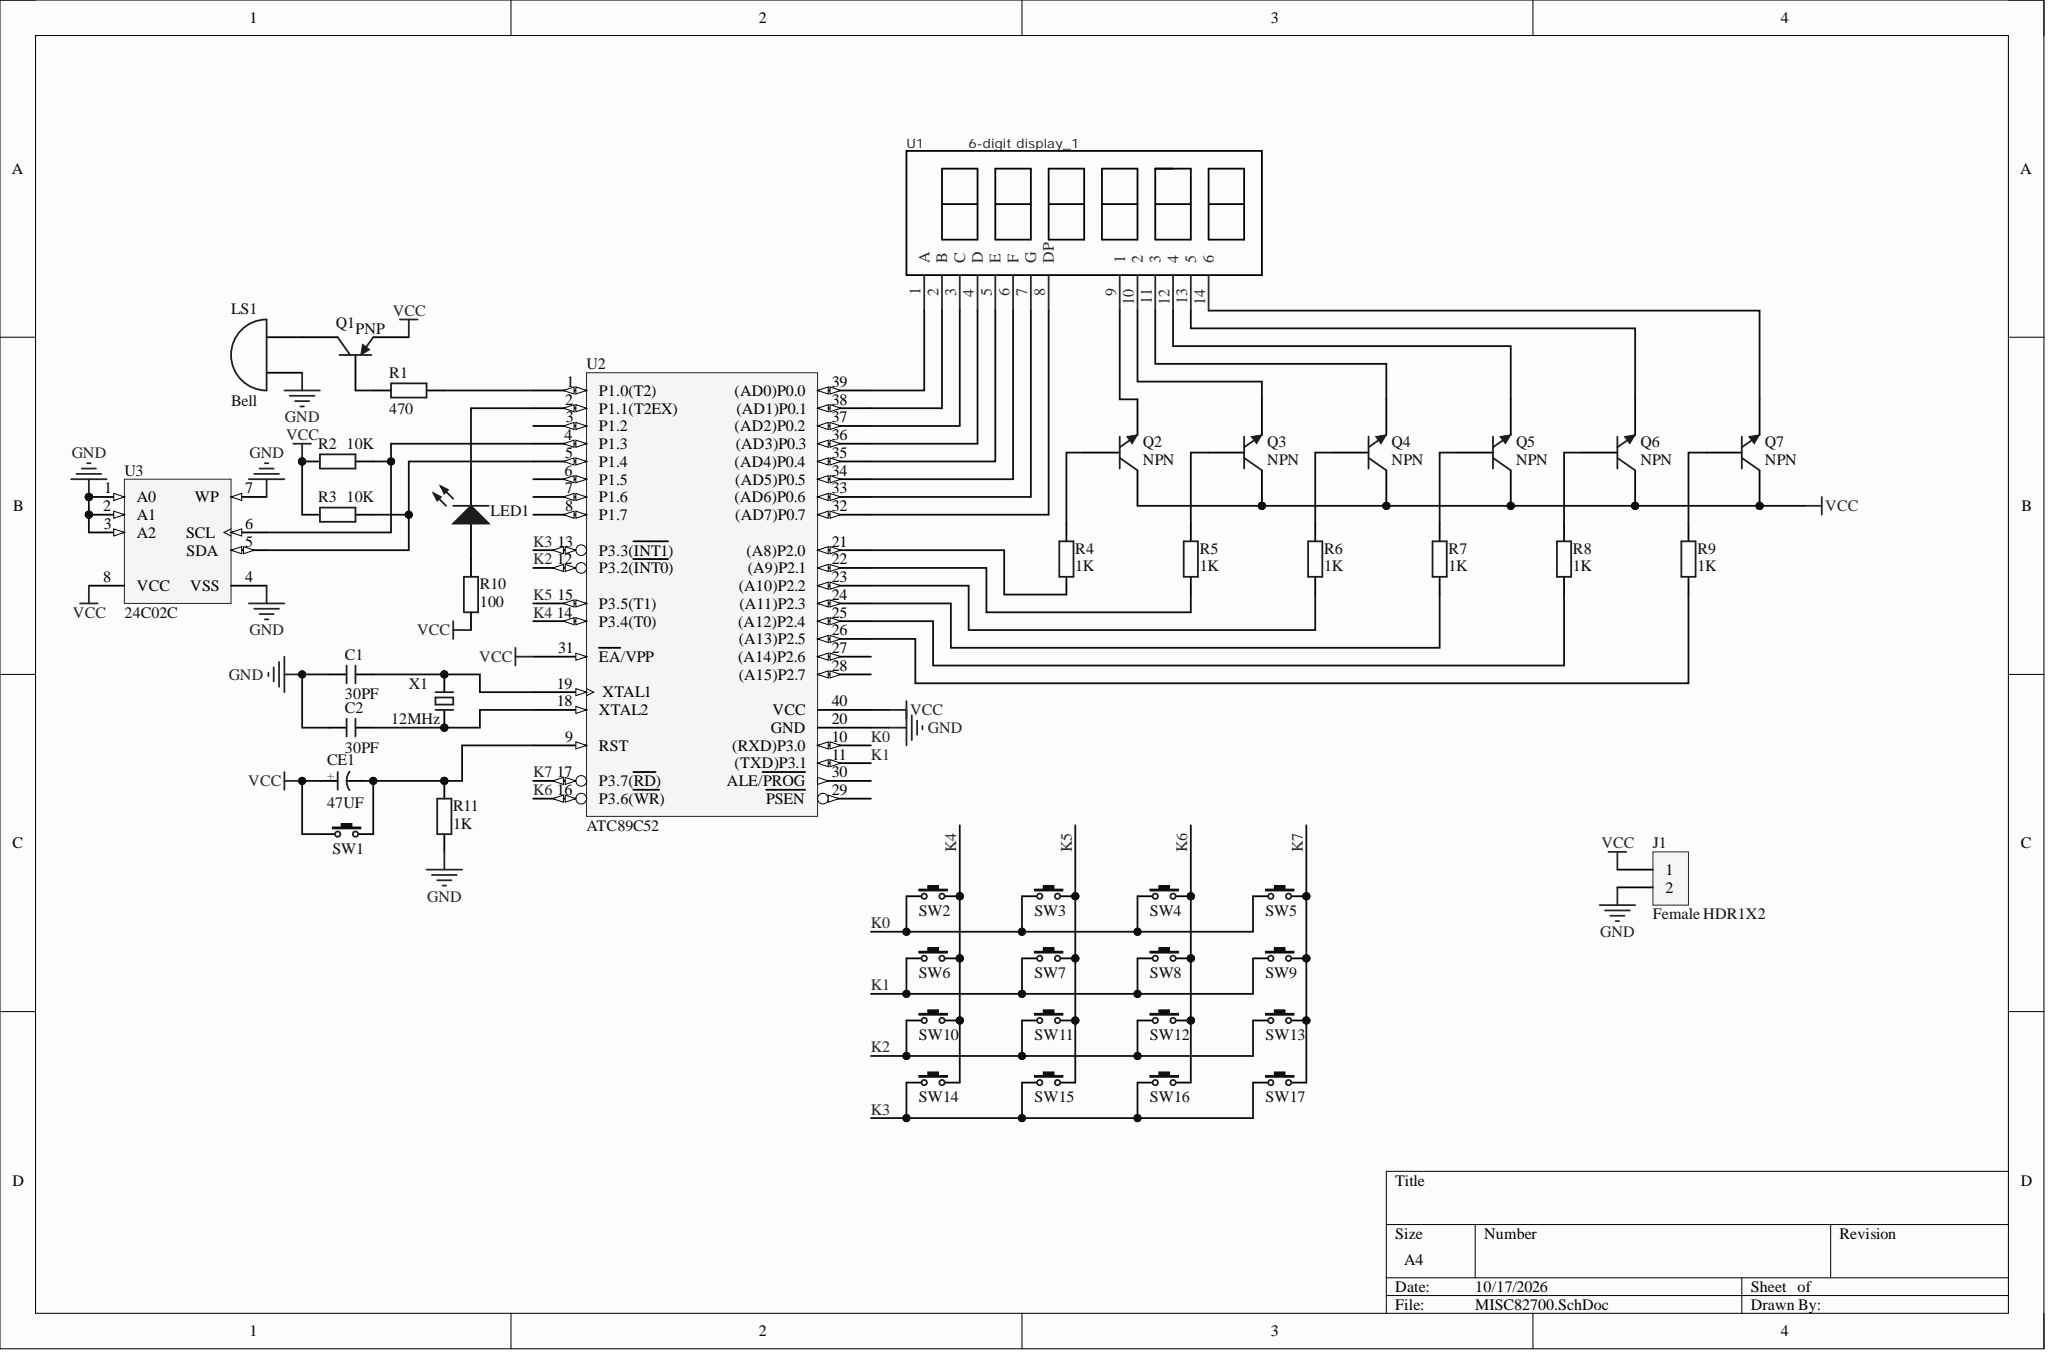Circuit board | Altium Designer | 45 parts | 46 nets
Bill of materials:
Comment,Description,Designator,Footprint,LibRef,Quantity
"30PF","Ceramic capacitor","C1, C2","CC 1.8*3.6","CC","2"
"47UF","Through-hole electrolytic capacitor","CE1","CAP 1.5*4*8","CE","1"
"Female HDR1X2","","J1","Fe-HDR1X2/2.54-S","Female HDR1X2","1"
"Red","5mm through-hole LED","LED1","LED 5MM-B","LED-5MM","1"
"Bell","Electrical Bell","LS1","PIN2","Bell","1"
"PNP","PNP General Purpose Amplifier","Q1","TO-92A","2N3906","1"
"NPN","NPN Bipolar Transistor","Q2, Q3, Q4, Q5, Q6, Q7","TO-226-AA","NPN","6"
"470","Color-band resistor","R1","RS 1/4W","R-S","1"
"10K","Color-band resistor","R2, R3","RS 1/4W","R-S","2"
"1K","Color-band resistor","R4, R5, R6, R7, R8, R9, R11","RS 1/4W","R-S","7"
"100","Color-band resistor","R10","RS 1/4W","R-S","1"
"3x6x5","3x6 tactile switch","SW1, SW2, SW3, SW4, SW5, SW6, SW7, SW8, SW9, SW10, SW11, SW12, SW13, SW14, SW15, SW16, SW17","四脚轻触开关","TSW 3x6","17"
"6-digit display_1","","U1","6位数码管","6位数码管_1","1"
"ATC89C52","","U2","DIP40","STC89C52","1"
"24C02C","2Kbit, 400kHz, 5V, I2C Serial EEPROM, 8-Pin PDIP, Industrial Temperature","U3","PDIP300-P8","24C02C-I/P","1"
"12MHz","2-pin passive crystal","X1","OSC HC-49S","XTAL-2P","1"
Netlist (Protel format):
[
C1
CC 1.8*3.6
30PF



]
[
C2
CC 1.8*3.6
30PF



]
[
CE1
CAP 1.5*4*8
47UF



]
[
J1
Fe-HDR1X2/2.54-S
Female HDR1X2



]
[
LED1
LED 5MM-B
Red



]
[
LS1
PIN2
Bell



]
[
Q1
TO-92A
PNP



]
[
Q2
TO-226-AA
NPN



]
[
Q3
TO-226-AA
NPN



]
[
Q4
TO-226-AA
NPN



]
[
Q5
TO-226-AA
NPN



]
[
Q6
TO-226-AA
NPN



]
[
Q7
TO-226-AA
NPN



]
[
R1
RS 1/4W
470



]
[
R2
RS 1/4W
10K



]
[
R3
RS 1/4W
10K



]
[
R4
RS 1/4W
1K



]
[
R5
RS 1/4W
1K



]
[
R6
RS 1/4W
1K



]
[
R7
RS 1/4W
1K



]
[
R8
RS 1/4W
1K



]
[
R9
RS 1/4W
1K



]
[
R10
RS 1/4W
100



]
[
R11
RS 1/4W
1K



]
[
SW1
四脚轻触开关
3x6x5



]
[
SW2
四脚轻触开关
3x6x5



]
[
SW3
四脚轻触开关
3x6x5



]
[
SW4
四脚轻触开关
3x6x5



]
[
SW5
四脚轻触开关
3x6x5



]
[
SW6
四脚轻触开关
3x6x5



]
[
SW7
四脚轻触开关
3x6x5



]
[
SW8
四脚轻触开关
3x6x5



]
[
SW9
四脚轻触开关
3x6x5



]
[
SW10
四脚轻触开关
3x6x5



]
[
SW11
四脚轻触开关
3x6x5



]
[
SW12
四脚轻触开关
3x6x5



]
[
SW13
四脚轻触开关
3x6x5



]
[
SW14
四脚轻触开关
3x6x5



]
[
SW15
四脚轻触开关
3x6x5



]
[
SW16
四脚轻触开关
3x6x5



]
[
SW17
四脚轻触开关
3x6x5



]
[
U1
6位数码管
6-digit display_1



]
[
U2
DIP40
ATC89C52



]
[
U3
PDIP300-P8
24C02C



]
[
X1
OSC HC-49S
12MHz



]
(
VCC
CE1-1
J1-1
Q1-1
Q2-1
Q3-1
Q4-1
Q5-1
Q6-1
Q7-1
R2-2
R3-2
R10-2
SW1-1
U2-31
U2-40
U3-8
)
(
NetU1_8
U1-8
U2-32
)
(
NetU1_7
U1-7
U2-33
)
(
NetU1_6
U1-6
U2-34
)
(
NetU1_5
U1-5
U2-35
)
(
NetU1_4
U1-4
U2-36
)
(
NetU1_3
U1-3
U2-37
)
(
NetU1_2
U1-2
U2-38
)
(
NetU1_1
U1-1
U2-39
)
(
NetR9_1
R9-1
U2-26
)
(
NetR8_1
R8-1
U2-25
)
(
NetR7_1
R7-1
U2-24
)
(
NetR6_1
R6-1
U2-23
)
(
NetR5_1
R5-1
U2-22
)
(
NetR4_1
R4-1
U2-21
)
(
NetR3_1
R3-1
U2-5
U3-5
)
(
NetR2_1
R2-1
U2-4
U3-6
)
(
NetR1_1
R1-1
U2-1
)
(
NetQ7_3
Q7-3
U1-14
)
(
NetQ7_2
Q7-2
R9-2
)
(
NetQ6_3
Q6-3
U1-13
)
(
NetQ6_2
Q6-2
R8-2
)
(
NetQ5_3
Q5-3
U1-12
)
(
NetQ5_2
Q5-2
R7-2
)
(
NetQ4_3
Q4-3
U1-11
)
(
NetQ4_2
Q4-2
R6-2
)
(
NetQ3_3
Q3-3
U1-10
)
(
NetQ3_2
Q3-2
R5-2
)
(
NetQ2_3
Q2-3
U1-9
)
(
NetQ2_2
Q2-2
R4-2
)
(
NetQ1_2
Q1-2
R1-2
)
(
NetLS1_2
LS1-2
Q1-3
)
(
NetLED1_2
LED1-2
U2-2
)
(
NetLED1_1
LED1-1
R10-1
)
(
NetCE1_2
CE1-2
R11-2
SW1-2
U2-9
)
(
NetC2_2
C2-2
U2-18
X1-1
)
(
NetC1_2
C1-2
U2-19
X1-2
)
(
K7
SW5-2
SW9-2
SW13-2
SW17-2
U2-17
)
(
K6
SW4-2
SW8-2
SW12-2
SW16-2
U2-16
)
(
K5
SW3-2
SW7-2
SW11-2
SW15-2
U2-15
)
(
K4
SW2-2
SW6-2
SW10-2
SW14-2
U2-14
)
(
K3
SW14-1
SW15-1
SW16-1
SW17-1
U2-13
)
(
K2
SW10-1
SW11-1
SW12-1
SW13-1
U2-12
)
(
K1
SW6-1
SW7-1
SW8-1
SW9-1
U2-11
)
(
K0
SW2-1
SW3-1
SW4-1
SW5-1
U2-10
)
(
GND
C1-1
C2-1
J1-2
LS1-1
R11-1
U2-20
U3-1
U3-2
U3-3
U3-4
U3-7
)